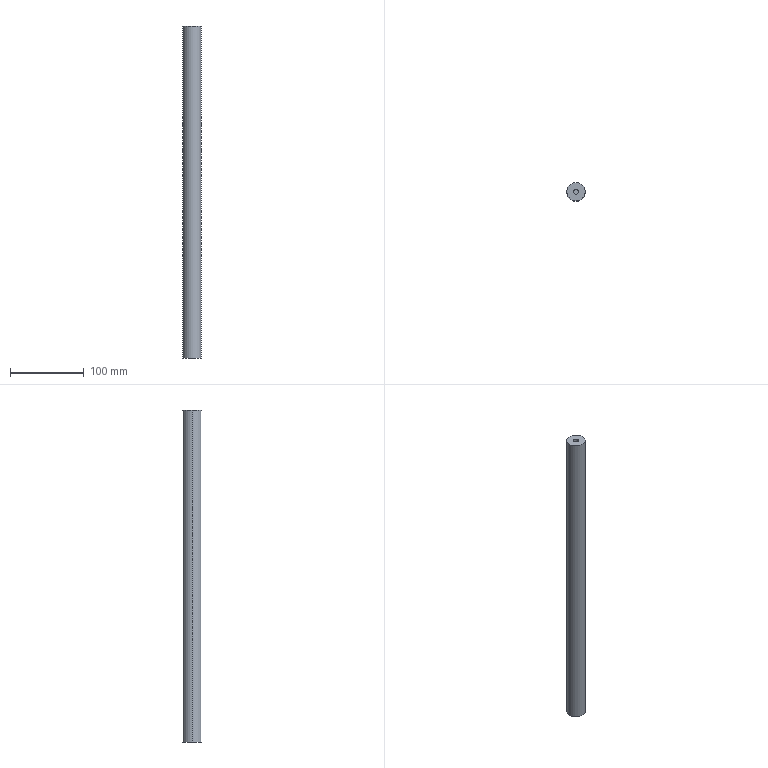Part | STEP file | 25 guide rod | 1 solid | 10 faces | box 25 x 25 x 450 mm | volume 219459 mm3 | cylinder 6 | plane 4 | commonest cylinder face diameters 6.8 x4 25 x2
STEP:
#1=CARTESIAN_POINT('',(0.,0.,0.));
#2=DIRECTION('',(0.,0.,1.));
#3=DIRECTION('',(1.,0.,0.));
#4=AXIS2_PLACEMENT_3D('',#1,#2,#3);
#5=CARTESIAN_POINT('',(-12.5,0.,450.));
#6=VERTEX_POINT('',#5);
#7=CARTESIAN_POINT('',(12.5,0.,450.));
#8=VERTEX_POINT('',#7);
#9=CARTESIAN_POINT('',(0.,0.,450.));
#10=DIRECTION('',(0.,0.,-1.));
#11=DIRECTION('',(-1.,0.,0.));
#12=AXIS2_PLACEMENT_3D('',#9,#10,#11);
#13=CIRCLE('',#12,12.5);
#14=CARTESIAN_POINT('',(0.,0.,450.));
#15=DIRECTION('',(0.,0.,-1.));
#16=DIRECTION('',(-1.,0.,0.));
#17=AXIS2_PLACEMENT_3D('',#14,#15,#16);
#18=CYLINDRICAL_SURFACE('',#17,12.5);
#19=CARTESIAN_POINT('',(0.,0.));
#20=DIRECTION('',(1.,0.));
#21=VECTOR('',#20,1.);
#22=LINE('',#19,#21);
#23=(GEOMETRIC_REPRESENTATION_CONTEXT(2)PARAMETRIC_REPRESENTATION_CONTEXT()REPRESENTATION_CONTEXT('',''));
#24=DEFINITIONAL_REPRESENTATION('',(#22),#23);
#25=PCURVE('',#18,#24);
#26=CARTESIAN_POINT('',(0.,0.,450.));
#27=DIRECTION('',(0.,0.,1.));
#28=DIRECTION('',(1.,0.,0.));
#29=AXIS2_PLACEMENT_3D('',#26,#27,#28);
#30=PLANE('',#29);
#31=CARTESIAN_POINT('',(-12.5,0.));
#32=CARTESIAN_POINT('',(-12.5,21.651));
#33=CARTESIAN_POINT('',(6.25,10.825));
#34=CARTESIAN_POINT('',(25.,0.));
#35=CARTESIAN_POINT('',(6.25,-10.825));
#36=CARTESIAN_POINT('',(-12.5,-21.651));
#37=CARTESIAN_POINT('',(-12.5,0.));
#38=(BOUNDED_CURVE()B_SPLINE_CURVE(2,(#31,#32,#33,#34,#35,#36,#37),.UNSPECIFIED.,.T.,.F.)B_SPLINE_CURVE_WITH_KNOTS((1,2,2,2,2,1),(-2.094,0.,2.094,4.189,6.283,8.378),.UNSPECIFIED.)CURVE()GEOMETRIC_REPRESENTATION_ITEM()RATIONAL_B_SPLINE_CURVE((1.,0.5,1.,0.5,1.,0.5,1.))REPRESENTATION_ITEM(''));
#39=(GEOMETRIC_REPRESENTATION_CONTEXT(2)PARAMETRIC_REPRESENTATION_CONTEXT()REPRESENTATION_CONTEXT('',''));
#40=DEFINITIONAL_REPRESENTATION('',(#38),#39);
#41=PCURVE('',#30,#40);
#42=SURFACE_CURVE('',#13,(#25,#41),.PCURVE_S1.);
#43=EDGE_CURVE('',#6,#8,#42,.T.);
#44=ORIENTED_EDGE('',*,*,#43,.T.);
#45=CARTESIAN_POINT('',(12.5,0.,0.));
#46=VERTEX_POINT('',#45);
#47=CARTESIAN_POINT('',(12.5,0.,450.));
#48=DIRECTION('',(0.,0.,-1.));
#49=VECTOR('',#48,1.);
#50=LINE('',#47,#49);
#51=CARTESIAN_POINT('',(3.142,0.));
#52=DIRECTION('',(0.,1.));
#53=VECTOR('',#52,1.);
#54=LINE('',#51,#53);
#55=(GEOMETRIC_REPRESENTATION_CONTEXT(2)PARAMETRIC_REPRESENTATION_CONTEXT()REPRESENTATION_CONTEXT('',''));
#56=DEFINITIONAL_REPRESENTATION('',(#54),#55);
#57=PCURVE('',#18,#56);
#58=CARTESIAN_POINT('',(0.,0.,450.));
#59=DIRECTION('',(0.,0.,-1.));
#60=DIRECTION('',(-1.,0.,0.));
#61=AXIS2_PLACEMENT_3D('',#58,#59,#60);
#62=CYLINDRICAL_SURFACE('',#61,12.5);
#63=CARTESIAN_POINT('',(3.142,0.));
#64=DIRECTION('',(0.,1.));
#65=VECTOR('',#64,1.);
#66=LINE('',#63,#65);
#67=(GEOMETRIC_REPRESENTATION_CONTEXT(2)PARAMETRIC_REPRESENTATION_CONTEXT()REPRESENTATION_CONTEXT('',''));
#68=DEFINITIONAL_REPRESENTATION('',(#66),#67);
#69=PCURVE('',#62,#68);
#70=SURFACE_CURVE('',#50,(#57,#69),.PCURVE_S1.);
#71=EDGE_CURVE('',#8,#46,#70,.T.);
#72=ORIENTED_EDGE('',*,*,#71,.T.);
#73=CARTESIAN_POINT('',(-12.5,0.,0.));
#74=VERTEX_POINT('',#73);
#75=CARTESIAN_POINT('',(0.,0.,0.));
#76=DIRECTION('',(0.,0.,1.));
#77=DIRECTION('',(-1.,0.,0.));
#78=AXIS2_PLACEMENT_3D('',#75,#76,#77);
#79=CIRCLE('',#78,12.5);
#80=CARTESIAN_POINT('',(6.283,450.));
#81=DIRECTION('',(-1.,0.));
#82=VECTOR('',#81,1.);
#83=LINE('',#80,#82);
#84=(GEOMETRIC_REPRESENTATION_CONTEXT(2)PARAMETRIC_REPRESENTATION_CONTEXT()REPRESENTATION_CONTEXT('',''));
#85=DEFINITIONAL_REPRESENTATION('',(#83),#84);
#86=PCURVE('',#18,#85);
#87=CARTESIAN_POINT('',(0.,0.,0.));
#88=DIRECTION('',(0.,0.,1.));
#89=DIRECTION('',(1.,0.,0.));
#90=AXIS2_PLACEMENT_3D('',#87,#88,#89);
#91=PLANE('',#90);
#92=CARTESIAN_POINT('',(0.,0.));
#93=DIRECTION('',(-1.,0.));
#94=AXIS2_PLACEMENT_2D('',#92,#93);
#95=CIRCLE('',#94,12.5);
#96=(GEOMETRIC_REPRESENTATION_CONTEXT(2)PARAMETRIC_REPRESENTATION_CONTEXT()REPRESENTATION_CONTEXT('',''));
#97=DEFINITIONAL_REPRESENTATION('',(#95),#96);
#98=PCURVE('',#91,#97);
#99=SURFACE_CURVE('',#79,(#86,#98),.PCURVE_S1.);
#100=EDGE_CURVE('',#46,#74,#99,.T.);
#101=ORIENTED_EDGE('',*,*,#100,.T.);
#102=CARTESIAN_POINT('',(-12.5,0.,450.));
#103=DIRECTION('',(0.,0.,-1.));
#104=VECTOR('',#103,1.);
#105=LINE('',#102,#104);
#106=CARTESIAN_POINT('',(0.,0.));
#107=DIRECTION('',(0.,1.));
#108=VECTOR('',#107,1.);
#109=LINE('',#106,#108);
#110=(GEOMETRIC_REPRESENTATION_CONTEXT(2)PARAMETRIC_REPRESENTATION_CONTEXT()REPRESENTATION_CONTEXT('',''));
#111=DEFINITIONAL_REPRESENTATION('',(#109),#110);
#112=PCURVE('',#18,#111);
#113=CARTESIAN_POINT('',(6.283,0.));
#114=DIRECTION('',(0.,1.));
#115=VECTOR('',#114,1.);
#116=LINE('',#113,#115);
#117=(GEOMETRIC_REPRESENTATION_CONTEXT(2)PARAMETRIC_REPRESENTATION_CONTEXT()REPRESENTATION_CONTEXT('',''));
#118=DEFINITIONAL_REPRESENTATION('',(#116),#117);
#119=PCURVE('',#62,#118);
#120=SURFACE_CURVE('',#105,(#112,#119),.PCURVE_S1.);
#121=EDGE_CURVE('',#6,#74,#120,.T.);
#122=ORIENTED_EDGE('',*,*,#121,.F.);
#123=EDGE_LOOP('',(#44,#72,#101,#122));
#124=FACE_BOUND('',#123,.T.);
#125=ADVANCED_FACE('',(#124),#18,.T.);
#126=CARTESIAN_POINT('',(-3.4,0.,19.75));
#127=VERTEX_POINT('',#126);
#128=CARTESIAN_POINT('',(-3.4,0.,0.));
#129=VERTEX_POINT('',#128);
#130=CARTESIAN_POINT('',(-3.4,0.,0.));
#131=DIRECTION('',(0.,0.,-1.));
#132=VECTOR('',#131,1.);
#133=LINE('',#130,#132);
#134=CARTESIAN_POINT('',(0.,0.,0.));
#135=DIRECTION('',(0.,0.,-1.));
#136=DIRECTION('',(-1.,0.,0.));
#137=AXIS2_PLACEMENT_3D('',#134,#135,#136);
#138=CYLINDRICAL_SURFACE('',#137,3.4);
#139=CARTESIAN_POINT('',(6.283,0.));
#140=DIRECTION('',(0.,1.));
#141=VECTOR('',#140,1.);
#142=LINE('',#139,#141);
#143=(GEOMETRIC_REPRESENTATION_CONTEXT(2)PARAMETRIC_REPRESENTATION_CONTEXT()REPRESENTATION_CONTEXT('',''));
#144=DEFINITIONAL_REPRESENTATION('',(#142),#143);
#145=PCURVE('',#138,#144);
#146=CARTESIAN_POINT('',(0.,0.,0.));
#147=DIRECTION('',(0.,0.,-1.));
#148=DIRECTION('',(-1.,0.,0.));
#149=AXIS2_PLACEMENT_3D('',#146,#147,#148);
#150=CYLINDRICAL_SURFACE('',#149,3.4);
#151=CARTESIAN_POINT('',(0.,0.));
#152=DIRECTION('',(0.,1.));
#153=VECTOR('',#152,1.);
#154=LINE('',#151,#153);
#155=(GEOMETRIC_REPRESENTATION_CONTEXT(2)PARAMETRIC_REPRESENTATION_CONTEXT()REPRESENTATION_CONTEXT('',''));
#156=DEFINITIONAL_REPRESENTATION('',(#154),#155);
#157=PCURVE('',#150,#156);
#158=SURFACE_CURVE('',#133,(#145,#157),.PCURVE_S1.);
#159=EDGE_CURVE('',#127,#129,#158,.T.);
#160=ORIENTED_EDGE('',*,*,#159,.T.);
#161=CARTESIAN_POINT('',(3.4,0.,0.));
#162=VERTEX_POINT('',#161);
#163=CARTESIAN_POINT('',(0.,0.,0.));
#164=DIRECTION('',(0.,0.,-1.));
#165=DIRECTION('',(-1.,0.,0.));
#166=AXIS2_PLACEMENT_3D('',#163,#164,#165);
#167=CIRCLE('',#166,3.4);
#168=CARTESIAN_POINT('',(0.,0.));
#169=DIRECTION('',(1.,0.));
#170=VECTOR('',#169,1.);
#171=LINE('',#168,#170);
#172=(GEOMETRIC_REPRESENTATION_CONTEXT(2)PARAMETRIC_REPRESENTATION_CONTEXT()REPRESENTATION_CONTEXT('',''));
#173=DEFINITIONAL_REPRESENTATION('',(#171),#172);
#174=PCURVE('',#138,#173);
#175=CARTESIAN_POINT('',(-3.4,0.));
#176=CARTESIAN_POINT('',(-3.4,5.889));
#177=CARTESIAN_POINT('',(1.7,2.944));
#178=CARTESIAN_POINT('',(6.8,0.));
#179=CARTESIAN_POINT('',(1.7,-2.944));
#180=CARTESIAN_POINT('',(-3.4,-5.889));
#181=CARTESIAN_POINT('',(-3.4,0.));
#182=(BOUNDED_CURVE()B_SPLINE_CURVE(2,(#175,#176,#177,#178,#179,#180,#181),.UNSPECIFIED.,.T.,.F.)B_SPLINE_CURVE_WITH_KNOTS((1,2,2,2,2,1),(-2.094,0.,2.094,4.189,6.283,8.378),.UNSPECIFIED.)CURVE()GEOMETRIC_REPRESENTATION_ITEM()RATIONAL_B_SPLINE_CURVE((1.,0.5,1.,0.5,1.,0.5,1.))REPRESENTATION_ITEM(''));
#183=(GEOMETRIC_REPRESENTATION_CONTEXT(2)PARAMETRIC_REPRESENTATION_CONTEXT()REPRESENTATION_CONTEXT('',''));
#184=DEFINITIONAL_REPRESENTATION('',(#182),#183);
#185=PCURVE('',#91,#184);
#186=SURFACE_CURVE('',#167,(#174,#185),.PCURVE_S1.);
#187=EDGE_CURVE('',#162,#129,#186,.T.);
#188=ORIENTED_EDGE('',*,*,#187,.F.);
#189=CARTESIAN_POINT('',(3.4,0.,19.75));
#190=VERTEX_POINT('',#189);
#191=CARTESIAN_POINT('',(3.4,0.,0.));
#192=DIRECTION('',(0.,0.,-1.));
#193=VECTOR('',#192,1.);
#194=LINE('',#191,#193);
#195=CARTESIAN_POINT('',(3.142,0.));
#196=DIRECTION('',(0.,1.));
#197=VECTOR('',#196,1.);
#198=LINE('',#195,#197);
#199=(GEOMETRIC_REPRESENTATION_CONTEXT(2)PARAMETRIC_REPRESENTATION_CONTEXT()REPRESENTATION_CONTEXT('',''));
#200=DEFINITIONAL_REPRESENTATION('',(#198),#199);
#201=PCURVE('',#138,#200);
#202=CARTESIAN_POINT('',(3.142,0.));
#203=DIRECTION('',(0.,1.));
#204=VECTOR('',#203,1.);
#205=LINE('',#202,#204);
#206=(GEOMETRIC_REPRESENTATION_CONTEXT(2)PARAMETRIC_REPRESENTATION_CONTEXT()REPRESENTATION_CONTEXT('',''));
#207=DEFINITIONAL_REPRESENTATION('',(#205),#206);
#208=PCURVE('',#150,#207);
#209=SURFACE_CURVE('',#194,(#201,#208),.PCURVE_S1.);
#210=EDGE_CURVE('',#190,#162,#209,.T.);
#211=ORIENTED_EDGE('',*,*,#210,.F.);
#212=CARTESIAN_POINT('',(0.,0.,19.75));
#213=DIRECTION('',(0.,0.,-1.));
#214=DIRECTION('',(-1.,0.,0.));
#215=AXIS2_PLACEMENT_3D('',#212,#213,#214);
#216=CIRCLE('',#215,3.4);
#217=CARTESIAN_POINT('',(0.,-19.75));
#218=DIRECTION('',(1.,0.));
#219=VECTOR('',#218,1.);
#220=LINE('',#217,#219);
#221=(GEOMETRIC_REPRESENTATION_CONTEXT(2)PARAMETRIC_REPRESENTATION_CONTEXT()REPRESENTATION_CONTEXT('',''));
#222=DEFINITIONAL_REPRESENTATION('',(#220),#221);
#223=PCURVE('',#138,#222);
#224=CARTESIAN_POINT('',(0.,0.,19.75));
#225=DIRECTION('',(0.,0.,1.));
#226=DIRECTION('',(1.,0.,0.));
#227=AXIS2_PLACEMENT_3D('',#224,#225,#226);
#228=PLANE('',#227);
#229=CARTESIAN_POINT('',(-3.4,0.));
#230=CARTESIAN_POINT('',(-3.4,5.889));
#231=CARTESIAN_POINT('',(1.7,2.944));
#232=CARTESIAN_POINT('',(6.8,0.));
#233=CARTESIAN_POINT('',(1.7,-2.944));
#234=CARTESIAN_POINT('',(-3.4,-5.889));
#235=CARTESIAN_POINT('',(-3.4,0.));
#236=(BOUNDED_CURVE()B_SPLINE_CURVE(2,(#229,#230,#231,#232,#233,#234,#235),.UNSPECIFIED.,.T.,.F.)B_SPLINE_CURVE_WITH_KNOTS((1,2,2,2,2,1),(-2.094,0.,2.094,4.189,6.283,8.378),.UNSPECIFIED.)CURVE()GEOMETRIC_REPRESENTATION_ITEM()RATIONAL_B_SPLINE_CURVE((1.,0.5,1.,0.5,1.,0.5,1.))REPRESENTATION_ITEM(''));
#237=(GEOMETRIC_REPRESENTATION_CONTEXT(2)PARAMETRIC_REPRESENTATION_CONTEXT()REPRESENTATION_CONTEXT('',''));
#238=DEFINITIONAL_REPRESENTATION('',(#236),#237);
#239=PCURVE('',#228,#238);
#240=SURFACE_CURVE('',#216,(#223,#239),.PCURVE_S1.);
#241=EDGE_CURVE('',#190,#127,#240,.T.);
#242=ORIENTED_EDGE('',*,*,#241,.T.);
#243=EDGE_LOOP('',(#160,#188,#211,#242));
#244=FACE_BOUND('',#243,.F.);
#245=ADVANCED_FACE('',(#244),#138,.F.);
#246=CARTESIAN_POINT('',(3.4,0.,430.25));
#247=VERTEX_POINT('',#246);
#248=CARTESIAN_POINT('',(3.4,0.,450.));
#249=VERTEX_POINT('',#248);
#250=CARTESIAN_POINT('',(3.4,0.,450.));
#251=DIRECTION('',(0.,0.,1.));
#252=VECTOR('',#251,1.);
#253=LINE('',#250,#252);
#254=CARTESIAN_POINT('',(0.,0.,450.));
#255=DIRECTION('',(0.,0.,1.));
#256=DIRECTION('',(1.,0.,0.));
#257=AXIS2_PLACEMENT_3D('',#254,#255,#256);
#258=CYLINDRICAL_SURFACE('',#257,3.4);
#259=CARTESIAN_POINT('',(6.283,0.));
#260=DIRECTION('',(0.,1.));
#261=VECTOR('',#260,1.);
#262=LINE('',#259,#261);
#263=(GEOMETRIC_REPRESENTATION_CONTEXT(2)PARAMETRIC_REPRESENTATION_CONTEXT()REPRESENTATION_CONTEXT('',''));
#264=DEFINITIONAL_REPRESENTATION('',(#262),#263);
#265=PCURVE('',#258,#264);
#266=CARTESIAN_POINT('',(0.,0.,450.));
#267=DIRECTION('',(0.,0.,1.));
#268=DIRECTION('',(1.,0.,0.));
#269=AXIS2_PLACEMENT_3D('',#266,#267,#268);
#270=CYLINDRICAL_SURFACE('',#269,3.4);
#271=CARTESIAN_POINT('',(0.,0.));
#272=DIRECTION('',(0.,1.));
#273=VECTOR('',#272,1.);
#274=LINE('',#271,#273);
#275=(GEOMETRIC_REPRESENTATION_CONTEXT(2)PARAMETRIC_REPRESENTATION_CONTEXT()REPRESENTATION_CONTEXT('',''));
#276=DEFINITIONAL_REPRESENTATION('',(#274),#275);
#277=PCURVE('',#270,#276);
#278=SURFACE_CURVE('',#253,(#265,#277),.PCURVE_S1.);
#279=EDGE_CURVE('',#247,#249,#278,.T.);
#280=ORIENTED_EDGE('',*,*,#279,.T.);
#281=CARTESIAN_POINT('',(-3.4,0.,450.));
#282=VERTEX_POINT('',#281);
#283=CARTESIAN_POINT('',(0.,0.,450.));
#284=DIRECTION('',(0.,0.,-1.));
#285=DIRECTION('',(1.,0.,0.));
#286=AXIS2_PLACEMENT_3D('',#283,#284,#285);
#287=CIRCLE('',#286,3.4);
#288=CARTESIAN_POINT('',(6.283,0.));
#289=DIRECTION('',(-1.,0.));
#290=VECTOR('',#289,1.);
#291=LINE('',#288,#290);
#292=(GEOMETRIC_REPRESENTATION_CONTEXT(2)PARAMETRIC_REPRESENTATION_CONTEXT()REPRESENTATION_CONTEXT('',''));
#293=DEFINITIONAL_REPRESENTATION('',(#291),#292);
#294=PCURVE('',#258,#293);
#295=CARTESIAN_POINT('',(3.4,0.));
#296=CARTESIAN_POINT('',(3.4,-5.889));
#297=CARTESIAN_POINT('',(-1.7,-2.944));
#298=CARTESIAN_POINT('',(-6.8,0.));
#299=CARTESIAN_POINT('',(-1.7,2.944));
#300=CARTESIAN_POINT('',(3.4,5.889));
#301=CARTESIAN_POINT('',(3.4,0.));
#302=(BOUNDED_CURVE()B_SPLINE_CURVE(2,(#295,#296,#297,#298,#299,#300,#301),.UNSPECIFIED.,.T.,.F.)B_SPLINE_CURVE_WITH_KNOTS((1,2,2,2,2,1),(-2.094,0.,2.094,4.189,6.283,8.378),.UNSPECIFIED.)CURVE()GEOMETRIC_REPRESENTATION_ITEM()RATIONAL_B_SPLINE_CURVE((1.,0.5,1.,0.5,1.,0.5,1.))REPRESENTATION_ITEM(''));
#303=(GEOMETRIC_REPRESENTATION_CONTEXT(2)PARAMETRIC_REPRESENTATION_CONTEXT()REPRESENTATION_CONTEXT('',''));
#304=DEFINITIONAL_REPRESENTATION('',(#302),#303);
#305=PCURVE('',#30,#304);
#306=SURFACE_CURVE('',#287,(#294,#305),.PCURVE_S1.);
#307=EDGE_CURVE('',#249,#282,#306,.T.);
#308=ORIENTED_EDGE('',*,*,#307,.T.);
#309=CARTESIAN_POINT('',(-3.4,0.,430.25));
#310=VERTEX_POINT('',#309);
#311=CARTESIAN_POINT('',(-3.4,0.,450.));
#312=DIRECTION('',(0.,0.,1.));
#313=VECTOR('',#312,1.);
#314=LINE('',#311,#313);
#315=CARTESIAN_POINT('',(3.142,0.));
#316=DIRECTION('',(0.,1.));
#317=VECTOR('',#316,1.);
#318=LINE('',#315,#317);
#319=(GEOMETRIC_REPRESENTATION_CONTEXT(2)PARAMETRIC_REPRESENTATION_CONTEXT()REPRESENTATION_CONTEXT('',''));
#320=DEFINITIONAL_REPRESENTATION('',(#318),#319);
#321=PCURVE('',#258,#320);
#322=CARTESIAN_POINT('',(3.142,0.));
#323=DIRECTION('',(0.,1.));
#324=VECTOR('',#323,1.);
#325=LINE('',#322,#324);
#326=(GEOMETRIC_REPRESENTATION_CONTEXT(2)PARAMETRIC_REPRESENTATION_CONTEXT()REPRESENTATION_CONTEXT('',''));
#327=DEFINITIONAL_REPRESENTATION('',(#325),#326);
#328=PCURVE('',#270,#327);
#329=SURFACE_CURVE('',#314,(#321,#328),.PCURVE_S1.);
#330=EDGE_CURVE('',#310,#282,#329,.T.);
#331=ORIENTED_EDGE('',*,*,#330,.F.);
#332=CARTESIAN_POINT('',(0.,0.,430.25));
#333=DIRECTION('',(0.,0.,1.));
#334=DIRECTION('',(1.,0.,0.));
#335=AXIS2_PLACEMENT_3D('',#332,#333,#334);
#336=CIRCLE('',#335,3.4);
#337=CARTESIAN_POINT('',(0.,-19.75));
#338=DIRECTION('',(1.,0.));
#339=VECTOR('',#338,1.);
#340=LINE('',#337,#339);
#341=(GEOMETRIC_REPRESENTATION_CONTEXT(2)PARAMETRIC_REPRESENTATION_CONTEXT()REPRESENTATION_CONTEXT('',''));
#342=DEFINITIONAL_REPRESENTATION('',(#340),#341);
#343=PCURVE('',#258,#342);
#344=CARTESIAN_POINT('',(0.,0.,430.25));
#345=DIRECTION('',(0.,0.,-1.));
#346=DIRECTION('',(-1.,0.,0.));
#347=AXIS2_PLACEMENT_3D('',#344,#345,#346);
#348=PLANE('',#347);
#349=CARTESIAN_POINT('',(-3.4,0.));
#350=CARTESIAN_POINT('',(-3.4,5.889));
#351=CARTESIAN_POINT('',(1.7,2.944));
#352=CARTESIAN_POINT('',(6.8,0.));
#353=CARTESIAN_POINT('',(1.7,-2.944));
#354=CARTESIAN_POINT('',(-3.4,-5.889));
#355=CARTESIAN_POINT('',(-3.4,0.));
#356=(BOUNDED_CURVE()B_SPLINE_CURVE(2,(#349,#350,#351,#352,#353,#354,#355),.UNSPECIFIED.,.T.,.F.)B_SPLINE_CURVE_WITH_KNOTS((1,2,2,2,2,1),(-2.094,0.,2.094,4.189,6.283,8.378),.UNSPECIFIED.)CURVE()GEOMETRIC_REPRESENTATION_ITEM()RATIONAL_B_SPLINE_CURVE((1.,0.5,1.,0.5,1.,0.5,1.))REPRESENTATION_ITEM(''));
#357=(GEOMETRIC_REPRESENTATION_CONTEXT(2)PARAMETRIC_REPRESENTATION_CONTEXT()REPRESENTATION_CONTEXT('',''));
#358=DEFINITIONAL_REPRESENTATION('',(#356),#357);
#359=PCURVE('',#348,#358);
#360=SURFACE_CURVE('',#336,(#343,#359),.PCURVE_S1.);
#361=EDGE_CURVE('',#310,#247,#360,.T.);
#362=ORIENTED_EDGE('',*,*,#361,.T.);
#363=EDGE_LOOP('',(#280,#308,#331,#362));
#364=FACE_BOUND('',#363,.F.);
#365=ADVANCED_FACE('',(#364),#258,.F.);
#366=ORIENTED_EDGE('',*,*,#71,.F.);
#367=CARTESIAN_POINT('',(0.,0.,450.));
#368=DIRECTION('',(0.,0.,-1.));
#369=DIRECTION('',(-1.,0.,0.));
#370=AXIS2_PLACEMENT_3D('',#367,#368,#369);
#371=CIRCLE('',#370,12.5);
#372=CARTESIAN_POINT('',(0.,0.));
#373=DIRECTION('',(1.,0.));
#374=VECTOR('',#373,1.);
#375=LINE('',#372,#374);
#376=(GEOMETRIC_REPRESENTATION_CONTEXT(2)PARAMETRIC_REPRESENTATION_CONTEXT()REPRESENTATION_CONTEXT('',''));
#377=DEFINITIONAL_REPRESENTATION('',(#375),#376);
#378=PCURVE('',#62,#377);
#379=CARTESIAN_POINT('',(-12.5,0.));
#380=CARTESIAN_POINT('',(-12.5,21.651));
#381=CARTESIAN_POINT('',(6.25,10.825));
#382=CARTESIAN_POINT('',(25.,0.));
#383=CARTESIAN_POINT('',(6.25,-10.825));
#384=CARTESIAN_POINT('',(-12.5,-21.651));
#385=CARTESIAN_POINT('',(-12.5,0.));
#386=(BOUNDED_CURVE()B_SPLINE_CURVE(2,(#379,#380,#381,#382,#383,#384,#385),.UNSPECIFIED.,.T.,.F.)B_SPLINE_CURVE_WITH_KNOTS((1,2,2,2,2,1),(-2.094,0.,2.094,4.189,6.283,8.378),.UNSPECIFIED.)CURVE()GEOMETRIC_REPRESENTATION_ITEM()RATIONAL_B_SPLINE_CURVE((1.,0.5,1.,0.5,1.,0.5,1.))REPRESENTATION_ITEM(''));
#387=(GEOMETRIC_REPRESENTATION_CONTEXT(2)PARAMETRIC_REPRESENTATION_CONTEXT()REPRESENTATION_CONTEXT('',''));
#388=DEFINITIONAL_REPRESENTATION('',(#386),#387);
#389=PCURVE('',#30,#388);
#390=SURFACE_CURVE('',#371,(#378,#389),.PCURVE_S1.);
#391=EDGE_CURVE('',#8,#6,#390,.T.);
#392=ORIENTED_EDGE('',*,*,#391,.T.);
#393=ORIENTED_EDGE('',*,*,#121,.T.);
#394=CARTESIAN_POINT('',(0.,0.,0.));
#395=DIRECTION('',(0.,0.,1.));
#396=DIRECTION('',(-1.,0.,0.));
#397=AXIS2_PLACEMENT_3D('',#394,#395,#396);
#398=CIRCLE('',#397,12.5);
#399=CARTESIAN_POINT('',(6.283,450.));
#400=DIRECTION('',(-1.,0.));
#401=VECTOR('',#400,1.);
#402=LINE('',#399,#401);
#403=(GEOMETRIC_REPRESENTATION_CONTEXT(2)PARAMETRIC_REPRESENTATION_CONTEXT()REPRESENTATION_CONTEXT('',''));
#404=DEFINITIONAL_REPRESENTATION('',(#402),#403);
#405=PCURVE('',#62,#404);
#406=CARTESIAN_POINT('',(0.,0.));
#407=DIRECTION('',(-1.,0.));
#408=AXIS2_PLACEMENT_2D('',#406,#407);
#409=CIRCLE('',#408,12.5);
#410=(GEOMETRIC_REPRESENTATION_CONTEXT(2)PARAMETRIC_REPRESENTATION_CONTEXT()REPRESENTATION_CONTEXT('',''));
#411=DEFINITIONAL_REPRESENTATION('',(#409),#410);
#412=PCURVE('',#91,#411);
#413=SURFACE_CURVE('',#398,(#405,#412),.PCURVE_S1.);
#414=EDGE_CURVE('',#74,#46,#413,.T.);
#415=ORIENTED_EDGE('',*,*,#414,.T.);
#416=EDGE_LOOP('',(#366,#392,#393,#415));
#417=FACE_BOUND('',#416,.T.);
#418=ADVANCED_FACE('',(#417),#62,.T.);
#419=ORIENTED_EDGE('',*,*,#414,.F.);
#420=ORIENTED_EDGE('',*,*,#100,.F.);
#421=EDGE_LOOP('',(#419,#420));
#422=FACE_BOUND('',#421,.T.);
#423=CARTESIAN_POINT('',(0.,0.,0.));
#424=DIRECTION('',(0.,0.,-1.));
#425=DIRECTION('',(-1.,0.,0.));
#426=AXIS2_PLACEMENT_3D('',#423,#424,#425);
#427=CIRCLE('',#426,3.4);
#428=CARTESIAN_POINT('',(-3.4,0.));
#429=CARTESIAN_POINT('',(-3.4,5.889));
#430=CARTESIAN_POINT('',(1.7,2.944));
#431=CARTESIAN_POINT('',(6.8,0.));
#432=CARTESIAN_POINT('',(1.7,-2.944));
#433=CARTESIAN_POINT('',(-3.4,-5.889));
#434=CARTESIAN_POINT('',(-3.4,0.));
#435=(BOUNDED_CURVE()B_SPLINE_CURVE(2,(#428,#429,#430,#431,#432,#433,#434),.UNSPECIFIED.,.T.,.F.)B_SPLINE_CURVE_WITH_KNOTS((1,2,2,2,2,1),(-2.094,0.,2.094,4.189,6.283,8.378),.UNSPECIFIED.)CURVE()GEOMETRIC_REPRESENTATION_ITEM()RATIONAL_B_SPLINE_CURVE((1.,0.5,1.,0.5,1.,0.5,1.))REPRESENTATION_ITEM(''));
#436=(GEOMETRIC_REPRESENTATION_CONTEXT(2)PARAMETRIC_REPRESENTATION_CONTEXT()REPRESENTATION_CONTEXT('',''));
#437=DEFINITIONAL_REPRESENTATION('',(#435),#436);
#438=PCURVE('',#91,#437);
#439=CARTESIAN_POINT('',(0.,0.));
#440=DIRECTION('',(1.,0.));
#441=VECTOR('',#440,1.);
#442=LINE('',#439,#441);
#443=(GEOMETRIC_REPRESENTATION_CONTEXT(2)PARAMETRIC_REPRESENTATION_CONTEXT()REPRESENTATION_CONTEXT('',''));
#444=DEFINITIONAL_REPRESENTATION('',(#442),#443);
#445=PCURVE('',#150,#444);
#446=SURFACE_CURVE('',#427,(#438,#445),.PCURVE_S1.);
#447=EDGE_CURVE('',#129,#162,#446,.T.);
#448=ORIENTED_EDGE('',*,*,#447,.F.);
#449=ORIENTED_EDGE('',*,*,#187,.F.);
#450=EDGE_LOOP('',(#448,#449));
#451=FACE_BOUND('',#450,.T.);
#452=ADVANCED_FACE('',(#422,#451),#91,.F.);
#453=ORIENTED_EDGE('',*,*,#43,.F.);
#454=ORIENTED_EDGE('',*,*,#391,.F.);
#455=EDGE_LOOP('',(#453,#454));
#456=FACE_BOUND('',#455,.T.);
#457=ORIENTED_EDGE('',*,*,#307,.T.);
#458=CARTESIAN_POINT('',(0.,0.,450.));
#459=DIRECTION('',(0.,0.,-1.));
#460=DIRECTION('',(1.,0.,0.));
#461=AXIS2_PLACEMENT_3D('',#458,#459,#460);
#462=CIRCLE('',#461,3.4);
#463=CARTESIAN_POINT('',(3.4,0.));
#464=CARTESIAN_POINT('',(3.4,-5.889));
#465=CARTESIAN_POINT('',(-1.7,-2.944));
#466=CARTESIAN_POINT('',(-6.8,0.));
#467=CARTESIAN_POINT('',(-1.7,2.944));
#468=CARTESIAN_POINT('',(3.4,5.889));
#469=CARTESIAN_POINT('',(3.4,0.));
#470=(BOUNDED_CURVE()B_SPLINE_CURVE(2,(#463,#464,#465,#466,#467,#468,#469),.UNSPECIFIED.,.T.,.F.)B_SPLINE_CURVE_WITH_KNOTS((1,2,2,2,2,1),(-2.094,0.,2.094,4.189,6.283,8.378),.UNSPECIFIED.)CURVE()GEOMETRIC_REPRESENTATION_ITEM()RATIONAL_B_SPLINE_CURVE((1.,0.5,1.,0.5,1.,0.5,1.))REPRESENTATION_ITEM(''));
#471=(GEOMETRIC_REPRESENTATION_CONTEXT(2)PARAMETRIC_REPRESENTATION_CONTEXT()REPRESENTATION_CONTEXT('',''));
#472=DEFINITIONAL_REPRESENTATION('',(#470),#471);
#473=PCURVE('',#30,#472);
#474=CARTESIAN_POINT('',(6.283,0.));
#475=DIRECTION('',(-1.,0.));
#476=VECTOR('',#475,1.);
#477=LINE('',#474,#476);
#478=(GEOMETRIC_REPRESENTATION_CONTEXT(2)PARAMETRIC_REPRESENTATION_CONTEXT()REPRESENTATION_CONTEXT('',''));
#479=DEFINITIONAL_REPRESENTATION('',(#477),#478);
#480=PCURVE('',#270,#479);
#481=SURFACE_CURVE('',#462,(#473,#480),.PCURVE_S1.);
#482=EDGE_CURVE('',#282,#249,#481,.T.);
#483=ORIENTED_EDGE('',*,*,#482,.T.);
#484=EDGE_LOOP('',(#457,#483));
#485=FACE_BOUND('',#484,.T.);
#486=ADVANCED_FACE('',(#456,#485),#30,.T.);
#487=ORIENTED_EDGE('',*,*,#447,.F.);
#488=ORIENTED_EDGE('',*,*,#159,.F.);
#489=CARTESIAN_POINT('',(0.,0.,19.75));
#490=DIRECTION('',(0.,0.,-1.));
#491=DIRECTION('',(-1.,0.,0.));
#492=AXIS2_PLACEMENT_3D('',#489,#490,#491);
#493=CIRCLE('',#492,3.4);
#494=CARTESIAN_POINT('',(0.,-19.75));
#495=DIRECTION('',(1.,0.));
#496=VECTOR('',#495,1.);
#497=LINE('',#494,#496);
#498=(GEOMETRIC_REPRESENTATION_CONTEXT(2)PARAMETRIC_REPRESENTATION_CONTEXT()REPRESENTATION_CONTEXT('',''));
#499=DEFINITIONAL_REPRESENTATION('',(#497),#498);
#500=PCURVE('',#150,#499);
#501=CARTESIAN_POINT('',(-3.4,0.));
#502=CARTESIAN_POINT('',(-3.4,5.889));
#503=CARTESIAN_POINT('',(1.7,2.944));
#504=CARTESIAN_POINT('',(6.8,0.));
#505=CARTESIAN_POINT('',(1.7,-2.944));
#506=CARTESIAN_POINT('',(-3.4,-5.889));
#507=CARTESIAN_POINT('',(-3.4,0.));
#508=(BOUNDED_CURVE()B_SPLINE_CURVE(2,(#501,#502,#503,#504,#505,#506,#507),.UNSPECIFIED.,.T.,.F.)B_SPLINE_CURVE_WITH_KNOTS((1,2,2,2,2,1),(-2.094,0.,2.094,4.189,6.283,8.378),.UNSPECIFIED.)CURVE()GEOMETRIC_REPRESENTATION_ITEM()RATIONAL_B_SPLINE_CURVE((1.,0.5,1.,0.5,1.,0.5,1.))REPRESENTATION_ITEM(''));
#509=(GEOMETRIC_REPRESENTATION_CONTEXT(2)PARAMETRIC_REPRESENTATION_CONTEXT()REPRESENTATION_CONTEXT('',''));
#510=DEFINITIONAL_REPRESENTATION('',(#508),#509);
#511=PCURVE('',#228,#510);
#512=SURFACE_CURVE('',#493,(#500,#511),.PCURVE_S1.);
#513=EDGE_CURVE('',#127,#190,#512,.T.);
#514=ORIENTED_EDGE('',*,*,#513,.T.);
#515=ORIENTED_EDGE('',*,*,#210,.T.);
#516=EDGE_LOOP('',(#487,#488,#514,#515));
#517=FACE_BOUND('',#516,.F.);
#518=ADVANCED_FACE('',(#517),#150,.F.);
#519=ORIENTED_EDGE('',*,*,#482,.T.);
#520=ORIENTED_EDGE('',*,*,#279,.F.);
#521=CARTESIAN_POINT('',(0.,0.,430.25));
#522=DIRECTION('',(0.,0.,1.));
#523=DIRECTION('',(1.,0.,0.));
#524=AXIS2_PLACEMENT_3D('',#521,#522,#523);
#525=CIRCLE('',#524,3.4);
#526=CARTESIAN_POINT('',(0.,-19.75));
#527=DIRECTION('',(1.,0.));
#528=VECTOR('',#527,1.);
#529=LINE('',#526,#528);
#530=(GEOMETRIC_REPRESENTATION_CONTEXT(2)PARAMETRIC_REPRESENTATION_CONTEXT()REPRESENTATION_CONTEXT('',''));
#531=DEFINITIONAL_REPRESENTATION('',(#529),#530);
#532=PCURVE('',#270,#531);
#533=CARTESIAN_POINT('',(-3.4,0.));
#534=CARTESIAN_POINT('',(-3.4,5.889));
#535=CARTESIAN_POINT('',(1.7,2.944));
#536=CARTESIAN_POINT('',(6.8,0.));
#537=CARTESIAN_POINT('',(1.7,-2.944));
#538=CARTESIAN_POINT('',(-3.4,-5.889));
#539=CARTESIAN_POINT('',(-3.4,0.));
#540=(BOUNDED_CURVE()B_SPLINE_CURVE(2,(#533,#534,#535,#536,#537,#538,#539),.UNSPECIFIED.,.T.,.F.)B_SPLINE_CURVE_WITH_KNOTS((1,2,2,2,2,1),(-2.094,0.,2.094,4.189,6.283,8.378),.UNSPECIFIED.)CURVE()GEOMETRIC_REPRESENTATION_ITEM()RATIONAL_B_SPLINE_CURVE((1.,0.5,1.,0.5,1.,0.5,1.))REPRESENTATION_ITEM(''));
#541=(GEOMETRIC_REPRESENTATION_CONTEXT(2)PARAMETRIC_REPRESENTATION_CONTEXT()REPRESENTATION_CONTEXT('',''));
#542=DEFINITIONAL_REPRESENTATION('',(#540),#541);
#543=PCURVE('',#348,#542);
#544=SURFACE_CURVE('',#525,(#532,#543),.PCURVE_S1.);
#545=EDGE_CURVE('',#247,#310,#544,.T.);
#546=ORIENTED_EDGE('',*,*,#545,.T.);
#547=ORIENTED_EDGE('',*,*,#330,.T.);
#548=EDGE_LOOP('',(#519,#520,#546,#547));
#549=FACE_BOUND('',#548,.F.);
#550=ADVANCED_FACE('',(#549),#270,.F.);
#551=ORIENTED_EDGE('',*,*,#513,.T.);
#552=ORIENTED_EDGE('',*,*,#241,.T.);
#553=EDGE_LOOP('',(#551,#552));
#554=FACE_BOUND('',#553,.T.);
#555=ADVANCED_FACE('',(#554),#228,.F.);
#556=ORIENTED_EDGE('',*,*,#545,.T.);
#557=ORIENTED_EDGE('',*,*,#361,.T.);
#558=EDGE_LOOP('',(#556,#557));
#559=FACE_BOUND('',#558,.T.);
#560=ADVANCED_FACE('',(#559),#348,.F.);
#561=CLOSED_SHELL('',(#125,#245,#365,#418,#452,#486,#518,#550,#555,#560));
#562=MANIFOLD_SOLID_BREP('',#561);
#563=(LENGTH_UNIT()NAMED_UNIT(*)SI_UNIT(.MILLI.,.METRE.));
#564=UNCERTAINTY_MEASURE_WITH_UNIT(LENGTH_MEASURE(0.0000001),#563,'','');
#565=(NAMED_UNIT(*)PLANE_ANGLE_UNIT()SI_UNIT($,.RADIAN.));
#566=(NAMED_UNIT(*)SI_UNIT($,.STERADIAN.)SOLID_ANGLE_UNIT());
#567=(GEOMETRIC_REPRESENTATION_CONTEXT(3)GLOBAL_UNCERTAINTY_ASSIGNED_CONTEXT((#564))GLOBAL_UNIT_ASSIGNED_CONTEXT((#563,#565,#566))REPRESENTATION_CONTEXT('',''));
#568=ADVANCED_BREP_SHAPE_REPRESENTATION('',(#4,#562),#567);